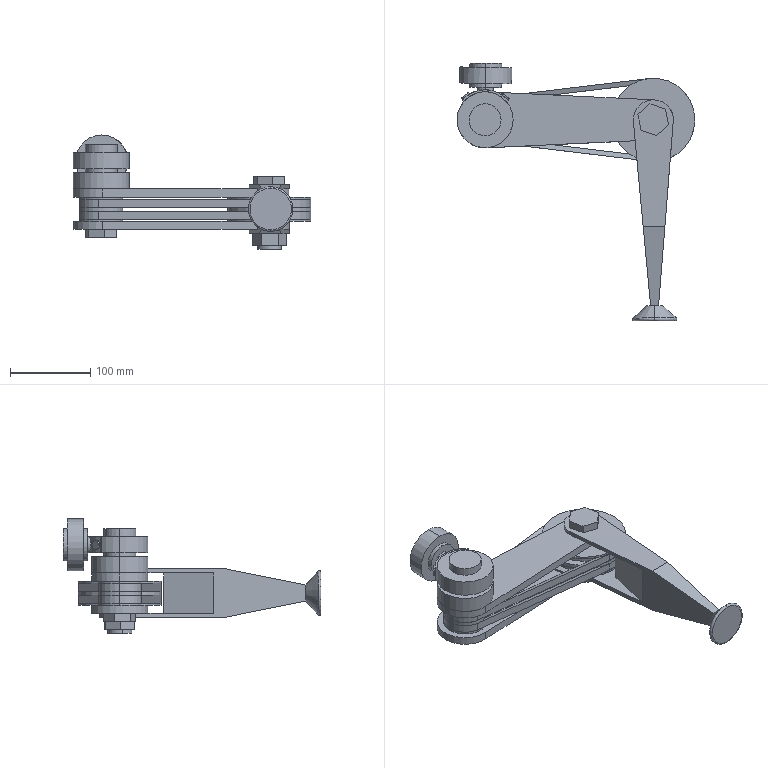Part | SolidWorks | features CompositeCurve 2 | 14 solids | 239 faces | box 297 x 321.802 x 142.5 mm | volume 1183355 mm3 | cylinder 107 | plane 104 | cone 18 | spline 8 | torus 2 | commonest cylinder face diameters 30 x20 10 x12 40 x12 70 x8 50 x7 54 x6